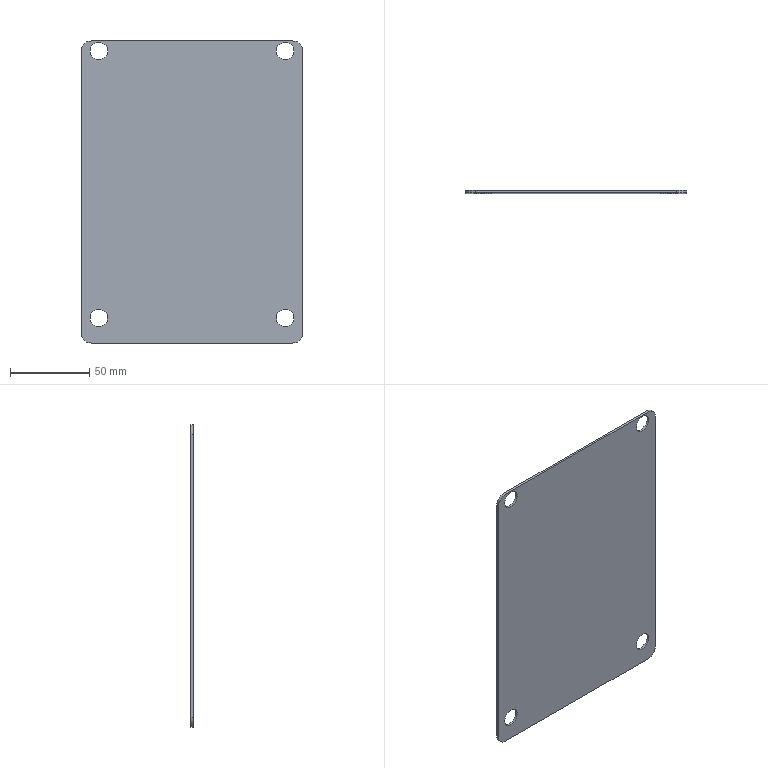Part | SolidWorks | features Extrusion 1, Fillet 1, HoleWzd 1, LPattern 1 | 1 solid | 18 faces | box 139.7 x 1.575 x 190.5 mm | volume 41244 mm3 | cylinder 12 | plane 6 | commonest cylinder face diameters 11.112 x8 12.7 x4
STEP:
#1=CARTESIAN_POINT('',(58.737,0.,78.581));
#2=VERTEX_POINT('',#1);
#3=CARTESIAN_POINT('',(58.737,0.,89.694));
#4=VERTEX_POINT('',#3);
#5=CARTESIAN_POINT('',(58.737,0.,84.138));
#6=DIRECTION('',(0.,1.,0.));
#7=DIRECTION('',(0.,0.,1.));
#8=AXIS2_PLACEMENT_3D('',#5,#6,#7);
#9=CIRCLE('',#8,5.556);
#10=EDGE_CURVE('',#2,#4,#9,.T.);
#11=ORIENTED_EDGE('',*,*,#10,.F.);
#12=CARTESIAN_POINT('',(58.737,1.575,78.581));
#13=VERTEX_POINT('',#12);
#14=CARTESIAN_POINT('',(58.737,1.575,78.581));
#15=DIRECTION('',(0.,1.,0.));
#16=VECTOR('',#15,1000.);
#17=LINE('',#14,#16);
#18=EDGE_CURVE('',#2,#13,#17,.T.);
#19=ORIENTED_EDGE('',*,*,#18,.T.);
#20=CARTESIAN_POINT('',(58.737,1.575,89.694));
#21=VERTEX_POINT('',#20);
#22=CARTESIAN_POINT('',(58.737,1.575,84.138));
#23=DIRECTION('',(0.,1.,0.));
#24=DIRECTION('',(0.,0.,1.));
#25=AXIS2_PLACEMENT_3D('',#22,#23,#24);
#26=CIRCLE('',#25,5.556);
#27=EDGE_CURVE('',#13,#21,#26,.T.);
#28=ORIENTED_EDGE('',*,*,#27,.T.);
#29=CARTESIAN_POINT('',(58.737,1.575,89.694));
#30=DIRECTION('',(0.,1.,0.));
#31=VECTOR('',#30,1000.);
#32=LINE('',#29,#31);
#33=EDGE_CURVE('',#4,#21,#32,.T.);
#34=ORIENTED_EDGE('',*,*,#33,.F.);
#35=EDGE_LOOP('',(#11,#19,#28,#34));
#36=FACE_OUTER_BOUND('',#35,.T.);
#37=CARTESIAN_POINT('',(58.737,1.575,84.138));
#38=DIRECTION('',(0.,1.,0.));
#39=DIRECTION('',(0.,0.,1.));
#40=AXIS2_PLACEMENT_3D('',#37,#38,#39);
#41=CYLINDRICAL_SURFACE('',#40,5.556);
#42=ADVANCED_FACE('',(#36),#41,.F.);
#43=CARTESIAN_POINT('',(-58.738,0.,78.581));
#44=VERTEX_POINT('',#43);
#45=CARTESIAN_POINT('',(-58.738,0.,89.694));
#46=VERTEX_POINT('',#45);
#47=CARTESIAN_POINT('',(-58.738,0.,84.138));
#48=DIRECTION('',(0.,1.,0.));
#49=DIRECTION('',(0.,0.,1.));
#50=AXIS2_PLACEMENT_3D('',#47,#48,#49);
#51=CIRCLE('',#50,5.556);
#52=EDGE_CURVE('',#44,#46,#51,.T.);
#53=ORIENTED_EDGE('',*,*,#52,.F.);
#54=CARTESIAN_POINT('',(-58.738,1.575,78.581));
#55=VERTEX_POINT('',#54);
#56=CARTESIAN_POINT('',(-58.738,1.575,78.581));
#57=DIRECTION('',(0.,1.,0.));
#58=VECTOR('',#57,1000.);
#59=LINE('',#56,#58);
#60=EDGE_CURVE('',#44,#55,#59,.T.);
#61=ORIENTED_EDGE('',*,*,#60,.T.);
#62=CARTESIAN_POINT('',(-58.738,1.575,89.694));
#63=VERTEX_POINT('',#62);
#64=CARTESIAN_POINT('',(-58.738,1.575,84.138));
#65=DIRECTION('',(0.,1.,0.));
#66=DIRECTION('',(0.,0.,1.));
#67=AXIS2_PLACEMENT_3D('',#64,#65,#66);
#68=CIRCLE('',#67,5.556);
#69=EDGE_CURVE('',#55,#63,#68,.T.);
#70=ORIENTED_EDGE('',*,*,#69,.T.);
#71=CARTESIAN_POINT('',(-58.738,1.575,89.694));
#72=DIRECTION('',(0.,1.,0.));
#73=VECTOR('',#72,1000.);
#74=LINE('',#71,#73);
#75=EDGE_CURVE('',#46,#63,#74,.T.);
#76=ORIENTED_EDGE('',*,*,#75,.F.);
#77=EDGE_LOOP('',(#53,#61,#70,#76));
#78=FACE_OUTER_BOUND('',#77,.T.);
#79=CARTESIAN_POINT('',(-58.738,1.575,84.138));
#80=DIRECTION('',(0.,1.,0.));
#81=DIRECTION('',(0.,0.,1.));
#82=AXIS2_PLACEMENT_3D('',#79,#80,#81);
#83=CYLINDRICAL_SURFACE('',#82,5.556);
#84=ADVANCED_FACE('',(#78),#83,.F.);
#85=CARTESIAN_POINT('',(58.737,0.,-89.694));
#86=VERTEX_POINT('',#85);
#87=CARTESIAN_POINT('',(58.737,0.,-78.581));
#88=VERTEX_POINT('',#87);
#89=CARTESIAN_POINT('',(58.737,0.,-84.138));
#90=DIRECTION('',(0.,1.,0.));
#91=DIRECTION('',(0.,0.,1.));
#92=AXIS2_PLACEMENT_3D('',#89,#90,#91);
#93=CIRCLE('',#92,5.556);
#94=EDGE_CURVE('',#86,#88,#93,.T.);
#95=ORIENTED_EDGE('',*,*,#94,.F.);
#96=CARTESIAN_POINT('',(58.737,1.575,-89.694));
#97=VERTEX_POINT('',#96);
#98=CARTESIAN_POINT('',(58.737,1.575,-89.694));
#99=DIRECTION('',(0.,1.,0.));
#100=VECTOR('',#99,1000.);
#101=LINE('',#98,#100);
#102=EDGE_CURVE('',#86,#97,#101,.T.);
#103=ORIENTED_EDGE('',*,*,#102,.T.);
#104=CARTESIAN_POINT('',(58.737,1.575,-78.581));
#105=VERTEX_POINT('',#104);
#106=CARTESIAN_POINT('',(58.737,1.575,-84.138));
#107=DIRECTION('',(0.,1.,0.));
#108=DIRECTION('',(0.,0.,1.));
#109=AXIS2_PLACEMENT_3D('',#106,#107,#108);
#110=CIRCLE('',#109,5.556);
#111=EDGE_CURVE('',#97,#105,#110,.T.);
#112=ORIENTED_EDGE('',*,*,#111,.T.);
#113=CARTESIAN_POINT('',(58.737,1.575,-78.581));
#114=DIRECTION('',(0.,1.,0.));
#115=VECTOR('',#114,1000.);
#116=LINE('',#113,#115);
#117=EDGE_CURVE('',#88,#105,#116,.T.);
#118=ORIENTED_EDGE('',*,*,#117,.F.);
#119=EDGE_LOOP('',(#95,#103,#112,#118));
#120=FACE_OUTER_BOUND('',#119,.T.);
#121=CARTESIAN_POINT('',(58.737,1.575,-84.138));
#122=DIRECTION('',(0.,1.,0.));
#123=DIRECTION('',(0.,0.,1.));
#124=AXIS2_PLACEMENT_3D('',#121,#122,#123);
#125=CYLINDRICAL_SURFACE('',#124,5.556);
#126=ADVANCED_FACE('',(#120),#125,.F.);
#127=CARTESIAN_POINT('',(-58.738,0.,-89.694));
#128=VERTEX_POINT('',#127);
#129=CARTESIAN_POINT('',(-58.738,0.,-78.581));
#130=VERTEX_POINT('',#129);
#131=CARTESIAN_POINT('',(-58.738,0.,-84.138));
#132=DIRECTION('',(0.,1.,0.));
#133=DIRECTION('',(0.,0.,1.));
#134=AXIS2_PLACEMENT_3D('',#131,#132,#133);
#135=CIRCLE('',#134,5.556);
#136=EDGE_CURVE('',#128,#130,#135,.T.);
#137=ORIENTED_EDGE('',*,*,#136,.F.);
#138=CARTESIAN_POINT('',(-58.738,1.575,-89.694));
#139=VERTEX_POINT('',#138);
#140=CARTESIAN_POINT('',(-58.738,1.575,-89.694));
#141=DIRECTION('',(0.,1.,0.));
#142=VECTOR('',#141,1000.);
#143=LINE('',#140,#142);
#144=EDGE_CURVE('',#128,#139,#143,.T.);
#145=ORIENTED_EDGE('',*,*,#144,.T.);
#146=CARTESIAN_POINT('',(-58.738,1.575,-78.581));
#147=VERTEX_POINT('',#146);
#148=CARTESIAN_POINT('',(-58.738,1.575,-84.138));
#149=DIRECTION('',(0.,1.,0.));
#150=DIRECTION('',(0.,0.,1.));
#151=AXIS2_PLACEMENT_3D('',#148,#149,#150);
#152=CIRCLE('',#151,5.556);
#153=EDGE_CURVE('',#139,#147,#152,.T.);
#154=ORIENTED_EDGE('',*,*,#153,.T.);
#155=CARTESIAN_POINT('',(-58.738,1.575,-78.581));
#156=DIRECTION('',(0.,1.,0.));
#157=VECTOR('',#156,1000.);
#158=LINE('',#155,#157);
#159=EDGE_CURVE('',#130,#147,#158,.T.);
#160=ORIENTED_EDGE('',*,*,#159,.F.);
#161=EDGE_LOOP('',(#137,#145,#154,#160));
#162=FACE_OUTER_BOUND('',#161,.T.);
#163=CARTESIAN_POINT('',(-58.738,1.575,-84.138));
#164=DIRECTION('',(0.,1.,0.));
#165=DIRECTION('',(0.,0.,1.));
#166=AXIS2_PLACEMENT_3D('',#163,#164,#165);
#167=CYLINDRICAL_SURFACE('',#166,5.556);
#168=ADVANCED_FACE('',(#162),#167,.F.);
#169=CARTESIAN_POINT('',(-69.85,1.575,-93.663));
#170=VERTEX_POINT('',#169);
#171=CARTESIAN_POINT('',(-69.85,1.575,84.138));
#172=VERTEX_POINT('',#171);
#173=CARTESIAN_POINT('',(-69.85,1.575,-100.013));
#174=DIRECTION('',(0.,0.,1.));
#175=VECTOR('',#174,1000.);
#176=LINE('',#173,#175);
#177=EDGE_CURVE('',#170,#172,#176,.T.);
#178=ORIENTED_EDGE('',*,*,#177,.F.);
#179=CARTESIAN_POINT('',(-69.85,0.,-93.663));
#180=VERTEX_POINT('',#179);
#181=CARTESIAN_POINT('',(-69.85,1.575,-93.663));
#182=DIRECTION('',(0.,-1.,0.));
#183=VECTOR('',#182,1000.);
#184=LINE('',#181,#183);
#185=EDGE_CURVE('',#170,#180,#184,.T.);
#186=ORIENTED_EDGE('',*,*,#185,.T.);
#187=CARTESIAN_POINT('',(-69.85,0.,84.138));
#188=VERTEX_POINT('',#187);
#189=CARTESIAN_POINT('',(-69.85,0.,-100.013));
#190=DIRECTION('',(0.,0.,1.));
#191=VECTOR('',#190,1000.);
#192=LINE('',#189,#191);
#193=EDGE_CURVE('',#180,#188,#192,.T.);
#194=ORIENTED_EDGE('',*,*,#193,.T.);
#195=CARTESIAN_POINT('',(-69.85,1.575,84.138));
#196=DIRECTION('',(0.,1.,0.));
#197=VECTOR('',#196,1000.);
#198=LINE('',#195,#197);
#199=EDGE_CURVE('',#188,#172,#198,.T.);
#200=ORIENTED_EDGE('',*,*,#199,.T.);
#201=EDGE_LOOP('',(#178,#186,#194,#200));
#202=FACE_OUTER_BOUND('',#201,.T.);
#203=CARTESIAN_POINT('',(-69.85,1.575,-100.013));
#204=DIRECTION('',(1.,0.,0.));
#205=DIRECTION('',(0.,0.,-1.));
#206=AXIS2_PLACEMENT_3D('',#203,#204,#205);
#207=PLANE('',#206);
#208=ADVANCED_FACE('',(#202),#207,.F.);
#209=CARTESIAN_POINT('',(-63.5,0.,90.487));
#210=VERTEX_POINT('',#209);
#211=CARTESIAN_POINT('',(63.5,0.,90.487));
#212=VERTEX_POINT('',#211);
#213=CARTESIAN_POINT('',(-69.85,0.,90.487));
#214=DIRECTION('',(1.,0.,0.));
#215=VECTOR('',#214,1000.);
#216=LINE('',#213,#215);
#217=EDGE_CURVE('',#210,#212,#216,.T.);
#218=ORIENTED_EDGE('',*,*,#217,.T.);
#219=CARTESIAN_POINT('',(63.5,1.575,90.487));
#220=VERTEX_POINT('',#219);
#221=CARTESIAN_POINT('',(63.5,1.575,90.487));
#222=DIRECTION('',(0.,1.,0.));
#223=VECTOR('',#222,1000.);
#224=LINE('',#221,#223);
#225=EDGE_CURVE('',#212,#220,#224,.T.);
#226=ORIENTED_EDGE('',*,*,#225,.T.);
#227=CARTESIAN_POINT('',(-63.5,1.575,90.487));
#228=VERTEX_POINT('',#227);
#229=CARTESIAN_POINT('',(-69.85,1.575,90.487));
#230=DIRECTION('',(1.,0.,0.));
#231=VECTOR('',#230,1000.);
#232=LINE('',#229,#231);
#233=EDGE_CURVE('',#228,#220,#232,.T.);
#234=ORIENTED_EDGE('',*,*,#233,.F.);
#235=CARTESIAN_POINT('',(-63.5,1.575,90.487));
#236=DIRECTION('',(0.,-1.,0.));
#237=VECTOR('',#236,1000.);
#238=LINE('',#235,#237);
#239=EDGE_CURVE('',#228,#210,#238,.T.);
#240=ORIENTED_EDGE('',*,*,#239,.T.);
#241=EDGE_LOOP('',(#218,#226,#234,#240));
#242=FACE_OUTER_BOUND('',#241,.T.);
#243=CARTESIAN_POINT('',(-69.85,1.575,90.487));
#244=DIRECTION('',(0.,0.,-1.));
#245=DIRECTION('',(-1.,0.,0.));
#246=AXIS2_PLACEMENT_3D('',#243,#244,#245);
#247=PLANE('',#246);
#248=ADVANCED_FACE('',(#242),#247,.F.);
#249=CARTESIAN_POINT('',(69.85,0.,84.138));
#250=VERTEX_POINT('',#249);
#251=CARTESIAN_POINT('',(69.85,0.,-93.663));
#252=VERTEX_POINT('',#251);
#253=CARTESIAN_POINT('',(69.85,0.,-100.013));
#254=DIRECTION('',(0.,0.,-1.));
#255=VECTOR('',#254,1000.);
#256=LINE('',#253,#255);
#257=EDGE_CURVE('',#250,#252,#256,.T.);
#258=ORIENTED_EDGE('',*,*,#257,.T.);
#259=CARTESIAN_POINT('',(69.85,1.575,-93.663));
#260=VERTEX_POINT('',#259);
#261=CARTESIAN_POINT('',(69.85,1.575,-93.663));
#262=DIRECTION('',(0.,1.,0.));
#263=VECTOR('',#262,1000.);
#264=LINE('',#261,#263);
#265=EDGE_CURVE('',#252,#260,#264,.T.);
#266=ORIENTED_EDGE('',*,*,#265,.T.);
#267=CARTESIAN_POINT('',(69.85,1.575,84.138));
#268=VERTEX_POINT('',#267);
#269=CARTESIAN_POINT('',(69.85,1.575,-100.013));
#270=DIRECTION('',(0.,0.,-1.));
#271=VECTOR('',#270,1000.);
#272=LINE('',#269,#271);
#273=EDGE_CURVE('',#268,#260,#272,.T.);
#274=ORIENTED_EDGE('',*,*,#273,.F.);
#275=CARTESIAN_POINT('',(69.85,1.575,84.138));
#276=DIRECTION('',(0.,-1.,0.));
#277=VECTOR('',#276,1000.);
#278=LINE('',#275,#277);
#279=EDGE_CURVE('',#268,#250,#278,.T.);
#280=ORIENTED_EDGE('',*,*,#279,.T.);
#281=EDGE_LOOP('',(#258,#266,#274,#280));
#282=FACE_OUTER_BOUND('',#281,.T.);
#283=CARTESIAN_POINT('',(69.85,1.575,-100.013));
#284=DIRECTION('',(-1.,0.,0.));
#285=DIRECTION('',(0.,0.,1.));
#286=AXIS2_PLACEMENT_3D('',#283,#284,#285);
#287=PLANE('',#286);
#288=ADVANCED_FACE('',(#282),#287,.F.);
#289=CARTESIAN_POINT('',(63.5,0.,-100.013));
#290=VERTEX_POINT('',#289);
#291=CARTESIAN_POINT('',(-63.5,0.,-100.013));
#292=VERTEX_POINT('',#291);
#293=CARTESIAN_POINT('',(-69.85,0.,-100.013));
#294=DIRECTION('',(-1.,0.,0.));
#295=VECTOR('',#294,1000.);
#296=LINE('',#293,#295);
#297=EDGE_CURVE('',#290,#292,#296,.T.);
#298=ORIENTED_EDGE('',*,*,#297,.T.);
#299=CARTESIAN_POINT('',(-63.5,1.575,-100.013));
#300=VERTEX_POINT('',#299);
#301=CARTESIAN_POINT('',(-63.5,1.575,-100.013));
#302=DIRECTION('',(0.,1.,0.));
#303=VECTOR('',#302,1000.);
#304=LINE('',#301,#303);
#305=EDGE_CURVE('',#292,#300,#304,.T.);
#306=ORIENTED_EDGE('',*,*,#305,.T.);
#307=CARTESIAN_POINT('',(63.5,1.575,-100.013));
#308=VERTEX_POINT('',#307);
#309=CARTESIAN_POINT('',(-69.85,1.575,-100.013));
#310=DIRECTION('',(-1.,0.,0.));
#311=VECTOR('',#310,1000.);
#312=LINE('',#309,#311);
#313=EDGE_CURVE('',#308,#300,#312,.T.);
#314=ORIENTED_EDGE('',*,*,#313,.F.);
#315=CARTESIAN_POINT('',(63.5,1.575,-100.013));
#316=DIRECTION('',(0.,-1.,0.));
#317=VECTOR('',#316,1000.);
#318=LINE('',#315,#317);
#319=EDGE_CURVE('',#308,#290,#318,.T.);
#320=ORIENTED_EDGE('',*,*,#319,.T.);
#321=EDGE_LOOP('',(#298,#306,#314,#320));
#322=FACE_OUTER_BOUND('',#321,.T.);
#323=CARTESIAN_POINT('',(-69.85,1.575,-100.013));
#324=DIRECTION('',(0.,0.,1.));
#325=DIRECTION('',(1.,0.,0.));
#326=AXIS2_PLACEMENT_3D('',#323,#324,#325);
#327=PLANE('',#326);
#328=ADVANCED_FACE('',(#322),#327,.F.);
#329=CARTESIAN_POINT('',(58.737,1.575,84.138));
#330=DIRECTION('',(0.,1.,0.));
#331=DIRECTION('',(0.,0.,1.));
#332=AXIS2_PLACEMENT_3D('',#329,#330,#331);
#333=CIRCLE('',#332,5.556);
#334=EDGE_CURVE('',#21,#13,#333,.T.);
#335=ORIENTED_EDGE('',*,*,#334,.F.);
#336=ORIENTED_EDGE('',*,*,#27,.F.);
#337=EDGE_LOOP('',(#335,#336));
#338=FACE_BOUND('',#337,.T.);
#339=CARTESIAN_POINT('',(-58.738,1.575,84.138));
#340=DIRECTION('',(0.,1.,0.));
#341=DIRECTION('',(0.,0.,1.));
#342=AXIS2_PLACEMENT_3D('',#339,#340,#341);
#343=CIRCLE('',#342,5.556);
#344=EDGE_CURVE('',#63,#55,#343,.T.);
#345=ORIENTED_EDGE('',*,*,#344,.F.);
#346=ORIENTED_EDGE('',*,*,#69,.F.);
#347=EDGE_LOOP('',(#345,#346));
#348=FACE_BOUND('',#347,.T.);
#349=CARTESIAN_POINT('',(58.737,1.575,-84.138));
#350=DIRECTION('',(0.,1.,0.));
#351=DIRECTION('',(0.,0.,1.));
#352=AXIS2_PLACEMENT_3D('',#349,#350,#351);
#353=CIRCLE('',#352,5.556);
#354=EDGE_CURVE('',#105,#97,#353,.T.);
#355=ORIENTED_EDGE('',*,*,#354,.F.);
#356=ORIENTED_EDGE('',*,*,#111,.F.);
#357=EDGE_LOOP('',(#355,#356));
#358=FACE_BOUND('',#357,.T.);
#359=CARTESIAN_POINT('',(-58.738,1.575,-84.138));
#360=DIRECTION('',(0.,1.,0.));
#361=DIRECTION('',(0.,0.,1.));
#362=AXIS2_PLACEMENT_3D('',#359,#360,#361);
#363=CIRCLE('',#362,5.556);
#364=EDGE_CURVE('',#147,#139,#363,.T.);
#365=ORIENTED_EDGE('',*,*,#364,.F.);
#366=ORIENTED_EDGE('',*,*,#153,.F.);
#367=EDGE_LOOP('',(#365,#366));
#368=FACE_BOUND('',#367,.T.);
#369=ORIENTED_EDGE('',*,*,#313,.T.);
#370=CARTESIAN_POINT('',(-63.5,1.575,-93.663));
#371=DIRECTION('',(0.,1.,0.));
#372=DIRECTION('',(0.,0.,1.));
#373=AXIS2_PLACEMENT_3D('',#370,#371,#372);
#374=CIRCLE('',#373,6.35);
#375=EDGE_CURVE('',#300,#170,#374,.T.);
#376=ORIENTED_EDGE('',*,*,#375,.T.);
#377=ORIENTED_EDGE('',*,*,#177,.T.);
#378=CARTESIAN_POINT('',(-63.5,1.575,84.138));
#379=DIRECTION('',(0.,1.,0.));
#380=DIRECTION('',(0.,0.,1.));
#381=AXIS2_PLACEMENT_3D('',#378,#379,#380);
#382=CIRCLE('',#381,6.35);
#383=EDGE_CURVE('',#172,#228,#382,.T.);
#384=ORIENTED_EDGE('',*,*,#383,.T.);
#385=ORIENTED_EDGE('',*,*,#233,.T.);
#386=CARTESIAN_POINT('',(63.5,1.575,84.138));
#387=DIRECTION('',(0.,1.,0.));
#388=DIRECTION('',(0.,0.,1.));
#389=AXIS2_PLACEMENT_3D('',#386,#387,#388);
#390=CIRCLE('',#389,6.35);
#391=EDGE_CURVE('',#220,#268,#390,.T.);
#392=ORIENTED_EDGE('',*,*,#391,.T.);
#393=ORIENTED_EDGE('',*,*,#273,.T.);
#394=CARTESIAN_POINT('',(63.5,1.575,-93.663));
#395=DIRECTION('',(0.,1.,0.));
#396=DIRECTION('',(0.,0.,1.));
#397=AXIS2_PLACEMENT_3D('',#394,#395,#396);
#398=CIRCLE('',#397,6.35);
#399=EDGE_CURVE('',#260,#308,#398,.T.);
#400=ORIENTED_EDGE('',*,*,#399,.T.);
#401=EDGE_LOOP('',(#369,#376,#377,#384,#385,#392,#393,#400));
#402=FACE_OUTER_BOUND('',#401,.T.);
#403=CARTESIAN_POINT('',(0.,1.575,0.));
#404=DIRECTION('',(0.,1.,0.));
#405=DIRECTION('',(0.,0.,1.));
#406=AXIS2_PLACEMENT_3D('',#403,#404,#405);
#407=PLANE('',#406);
#408=ADVANCED_FACE('',(#338,#348,#358,#368,#402),#407,.T.);
#409=CARTESIAN_POINT('',(58.737,0.,84.138));
#410=DIRECTION('',(0.,1.,0.));
#411=DIRECTION('',(0.,0.,1.));
#412=AXIS2_PLACEMENT_3D('',#409,#410,#411);
#413=CIRCLE('',#412,5.556);
#414=EDGE_CURVE('',#4,#2,#413,.T.);
#415=ORIENTED_EDGE('',*,*,#414,.T.);
#416=ORIENTED_EDGE('',*,*,#10,.T.);
#417=EDGE_LOOP('',(#415,#416));
#418=FACE_BOUND('',#417,.T.);
#419=CARTESIAN_POINT('',(-58.738,0.,84.138));
#420=DIRECTION('',(0.,1.,0.));
#421=DIRECTION('',(0.,0.,1.));
#422=AXIS2_PLACEMENT_3D('',#419,#420,#421);
#423=CIRCLE('',#422,5.556);
#424=EDGE_CURVE('',#46,#44,#423,.T.);
#425=ORIENTED_EDGE('',*,*,#424,.T.);
#426=ORIENTED_EDGE('',*,*,#52,.T.);
#427=EDGE_LOOP('',(#425,#426));
#428=FACE_BOUND('',#427,.T.);
#429=CARTESIAN_POINT('',(58.737,0.,-84.138));
#430=DIRECTION('',(0.,1.,0.));
#431=DIRECTION('',(0.,0.,1.));
#432=AXIS2_PLACEMENT_3D('',#429,#430,#431);
#433=CIRCLE('',#432,5.556);
#434=EDGE_CURVE('',#88,#86,#433,.T.);
#435=ORIENTED_EDGE('',*,*,#434,.T.);
#436=ORIENTED_EDGE('',*,*,#94,.T.);
#437=EDGE_LOOP('',(#435,#436));
#438=FACE_BOUND('',#437,.T.);
#439=CARTESIAN_POINT('',(-58.738,0.,-84.138));
#440=DIRECTION('',(0.,1.,0.));
#441=DIRECTION('',(0.,0.,1.));
#442=AXIS2_PLACEMENT_3D('',#439,#440,#441);
#443=CIRCLE('',#442,5.556);
#444=EDGE_CURVE('',#130,#128,#443,.T.);
#445=ORIENTED_EDGE('',*,*,#444,.T.);
#446=ORIENTED_EDGE('',*,*,#136,.T.);
#447=EDGE_LOOP('',(#445,#446));
#448=FACE_BOUND('',#447,.T.);
#449=ORIENTED_EDGE('',*,*,#193,.F.);
#450=CARTESIAN_POINT('',(-63.5,0.,-93.663));
#451=DIRECTION('',(0.,-1.,0.));
#452=DIRECTION('',(0.,0.,1.));
#453=AXIS2_PLACEMENT_3D('',#450,#451,#452);
#454=CIRCLE('',#453,6.35);
#455=EDGE_CURVE('',#180,#292,#454,.T.);
#456=ORIENTED_EDGE('',*,*,#455,.T.);
#457=ORIENTED_EDGE('',*,*,#297,.F.);
#458=CARTESIAN_POINT('',(63.5,0.,-93.663));
#459=DIRECTION('',(0.,-1.,0.));
#460=DIRECTION('',(0.,0.,1.));
#461=AXIS2_PLACEMENT_3D('',#458,#459,#460);
#462=CIRCLE('',#461,6.35);
#463=EDGE_CURVE('',#290,#252,#462,.T.);
#464=ORIENTED_EDGE('',*,*,#463,.T.);
#465=ORIENTED_EDGE('',*,*,#257,.F.);
#466=CARTESIAN_POINT('',(63.5,0.,84.138));
#467=DIRECTION('',(0.,-1.,0.));
#468=DIRECTION('',(0.,0.,1.));
#469=AXIS2_PLACEMENT_3D('',#466,#467,#468);
#470=CIRCLE('',#469,6.35);
#471=EDGE_CURVE('',#250,#212,#470,.T.);
#472=ORIENTED_EDGE('',*,*,#471,.T.);
#473=ORIENTED_EDGE('',*,*,#217,.F.);
#474=CARTESIAN_POINT('',(-63.5,0.,84.138));
#475=DIRECTION('',(0.,-1.,0.));
#476=DIRECTION('',(0.,0.,1.));
#477=AXIS2_PLACEMENT_3D('',#474,#475,#476);
#478=CIRCLE('',#477,6.35);
#479=EDGE_CURVE('',#210,#188,#478,.T.);
#480=ORIENTED_EDGE('',*,*,#479,.T.);
#481=EDGE_LOOP('',(#449,#456,#457,#464,#465,#472,#473,#480));
#482=FACE_OUTER_BOUND('',#481,.T.);
#483=CARTESIAN_POINT('',(0.,0.,0.));
#484=DIRECTION('',(0.,1.,0.));
#485=DIRECTION('',(0.,0.,1.));
#486=AXIS2_PLACEMENT_3D('',#483,#484,#485);
#487=PLANE('',#486);
#488=ADVANCED_FACE('',(#418,#428,#438,#448,#482),#487,.F.);
#489=ORIENTED_EDGE('',*,*,#375,.F.);
#490=ORIENTED_EDGE('',*,*,#305,.F.);
#491=ORIENTED_EDGE('',*,*,#455,.F.);
#492=ORIENTED_EDGE('',*,*,#185,.F.);
#493=EDGE_LOOP('',(#489,#490,#491,#492));
#494=FACE_OUTER_BOUND('',#493,.T.);
#495=CARTESIAN_POINT('',(-63.5,1.575,-93.663));
#496=DIRECTION('',(0.,-1.,0.));
#497=DIRECTION('',(0.,0.,-1.));
#498=AXIS2_PLACEMENT_3D('',#495,#496,#497);
#499=CYLINDRICAL_SURFACE('',#498,6.35);
#500=ADVANCED_FACE('',(#494),#499,.T.);
#501=ORIENTED_EDGE('',*,*,#399,.F.);
#502=ORIENTED_EDGE('',*,*,#265,.F.);
#503=ORIENTED_EDGE('',*,*,#463,.F.);
#504=ORIENTED_EDGE('',*,*,#319,.F.);
#505=EDGE_LOOP('',(#501,#502,#503,#504));
#506=FACE_OUTER_BOUND('',#505,.T.);
#507=CARTESIAN_POINT('',(63.5,1.575,-93.663));
#508=DIRECTION('',(0.,-1.,0.));
#509=DIRECTION('',(0.,0.,-1.));
#510=AXIS2_PLACEMENT_3D('',#507,#508,#509);
#511=CYLINDRICAL_SURFACE('',#510,6.35);
#512=ADVANCED_FACE('',(#506),#511,.T.);
#513=ORIENTED_EDGE('',*,*,#391,.F.);
#514=ORIENTED_EDGE('',*,*,#225,.F.);
#515=ORIENTED_EDGE('',*,*,#471,.F.);
#516=ORIENTED_EDGE('',*,*,#279,.F.);
#517=EDGE_LOOP('',(#513,#514,#515,#516));
#518=FACE_OUTER_BOUND('',#517,.T.);
#519=CARTESIAN_POINT('',(63.5,1.575,84.138));
#520=DIRECTION('',(0.,-1.,0.));
#521=DIRECTION('',(0.,0.,-1.));
#522=AXIS2_PLACEMENT_3D('',#519,#520,#521);
#523=CYLINDRICAL_SURFACE('',#522,6.35);
#524=ADVANCED_FACE('',(#518),#523,.T.);
#525=ORIENTED_EDGE('',*,*,#383,.F.);
#526=ORIENTED_EDGE('',*,*,#199,.F.);
#527=ORIENTED_EDGE('',*,*,#479,.F.);
#528=ORIENTED_EDGE('',*,*,#239,.F.);
#529=EDGE_LOOP('',(#525,#526,#527,#528));
#530=FACE_OUTER_BOUND('',#529,.T.);
#531=CARTESIAN_POINT('',(-63.5,1.575,84.138));
#532=DIRECTION('',(0.,-1.,0.));
#533=DIRECTION('',(0.,0.,-1.));
#534=AXIS2_PLACEMENT_3D('',#531,#532,#533);
#535=CYLINDRICAL_SURFACE('',#534,6.35);
#536=ADVANCED_FACE('',(#530),#535,.T.);
#537=ORIENTED_EDGE('',*,*,#144,.F.);
#538=ORIENTED_EDGE('',*,*,#444,.F.);
#539=ORIENTED_EDGE('',*,*,#159,.T.);
#540=ORIENTED_EDGE('',*,*,#364,.T.);
#541=EDGE_LOOP('',(#537,#538,#539,#540));
#542=FACE_OUTER_BOUND('',#541,.T.);
#543=CARTESIAN_POINT('',(-58.738,1.575,-84.138));
#544=DIRECTION('',(0.,1.,0.));
#545=DIRECTION('',(0.,0.,1.));
#546=AXIS2_PLACEMENT_3D('',#543,#544,#545);
#547=CYLINDRICAL_SURFACE('',#546,5.556);
#548=ADVANCED_FACE('',(#542),#547,.F.);
#549=ORIENTED_EDGE('',*,*,#102,.F.);
#550=ORIENTED_EDGE('',*,*,#434,.F.);
#551=ORIENTED_EDGE('',*,*,#117,.T.);
#552=ORIENTED_EDGE('',*,*,#354,.T.);
#553=EDGE_LOOP('',(#549,#550,#551,#552));
#554=FACE_OUTER_BOUND('',#553,.T.);
#555=CARTESIAN_POINT('',(58.737,1.575,-84.138));
#556=DIRECTION('',(0.,1.,0.));
#557=DIRECTION('',(0.,0.,1.));
#558=AXIS2_PLACEMENT_3D('',#555,#556,#557);
#559=CYLINDRICAL_SURFACE('',#558,5.556);
#560=ADVANCED_FACE('',(#554),#559,.F.);
#561=ORIENTED_EDGE('',*,*,#60,.F.);
#562=ORIENTED_EDGE('',*,*,#424,.F.);
#563=ORIENTED_EDGE('',*,*,#75,.T.);
#564=ORIENTED_EDGE('',*,*,#344,.T.);
#565=EDGE_LOOP('',(#561,#562,#563,#564));
#566=FACE_OUTER_BOUND('',#565,.T.);
#567=CARTESIAN_POINT('',(-58.738,1.575,84.138));
#568=DIRECTION('',(0.,1.,0.));
#569=DIRECTION('',(0.,0.,1.));
#570=AXIS2_PLACEMENT_3D('',#567,#568,#569);
#571=CYLINDRICAL_SURFACE('',#570,5.556);
#572=ADVANCED_FACE('',(#566),#571,.F.);
#573=ORIENTED_EDGE('',*,*,#18,.F.);
#574=ORIENTED_EDGE('',*,*,#414,.F.);
#575=ORIENTED_EDGE('',*,*,#33,.T.);
#576=ORIENTED_EDGE('',*,*,#334,.T.);
#577=EDGE_LOOP('',(#573,#574,#575,#576));
#578=FACE_OUTER_BOUND('',#577,.T.);
#579=CARTESIAN_POINT('',(58.737,1.575,84.138));
#580=DIRECTION('',(0.,1.,0.));
#581=DIRECTION('',(0.,0.,1.));
#582=AXIS2_PLACEMENT_3D('',#579,#580,#581);
#583=CYLINDRICAL_SURFACE('',#582,5.556);
#584=ADVANCED_FACE('',(#578),#583,.F.);
#585=CLOSED_SHELL('',(#42,#84,#126,#168,#208,#248,#288,#328,#408,#488,#500,#512,#524,#536,#548,#560,#572,#584));
#586=MANIFOLD_SOLID_BREP('',#585);
#587=CARTESIAN_POINT('',(0.,0.,0.));
#588=DIRECTION('',(0.,0.,1.));
#589=DIRECTION('',(1.,0.,0.));
#590=AXIS2_PLACEMENT_3D('',#587,#588,#589);
#591=(LENGTH_UNIT()NAMED_UNIT(*)SI_UNIT(.MILLI.,.METRE.));
#592=UNCERTAINTY_MEASURE_WITH_UNIT(LENGTH_MEASURE(0.00001),#591,'','');
#593=(NAMED_UNIT(*)PLANE_ANGLE_UNIT()SI_UNIT($,.RADIAN.));
#594=(NAMED_UNIT(*)SI_UNIT($,.STERADIAN.)SOLID_ANGLE_UNIT());
#595=(GEOMETRIC_REPRESENTATION_CONTEXT(3)GLOBAL_UNCERTAINTY_ASSIGNED_CONTEXT((#592))GLOBAL_UNIT_ASSIGNED_CONTEXT((#591,#593,#594))REPRESENTATION_CONTEXT('',''));
#596=ADVANCED_BREP_SHAPE_REPRESENTATION('',(#586,#590),#595);